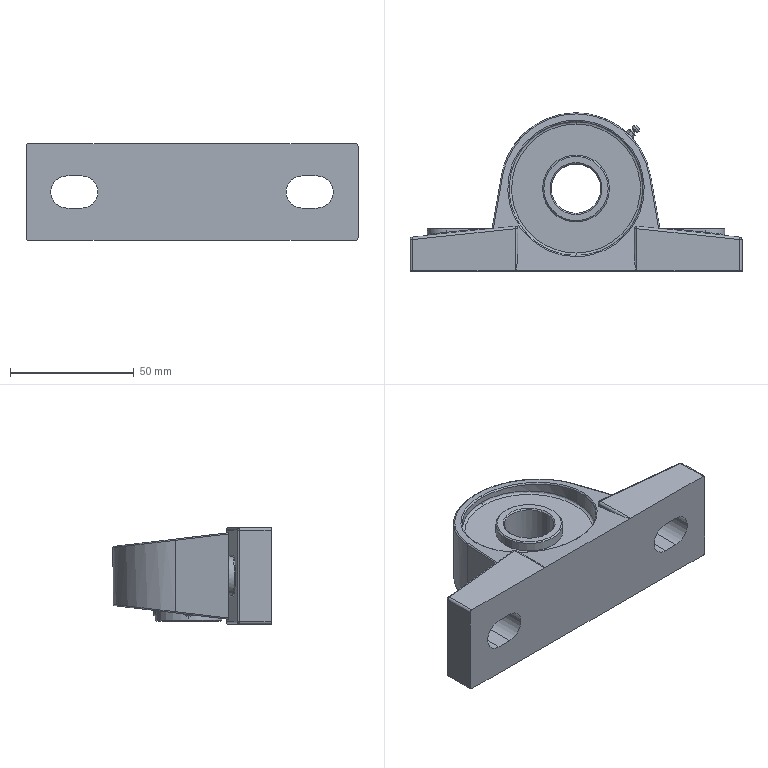Part | STEP file | 1 solid | 150 faces | box 134 x 63.85 x 39 mm | volume 118753 mm3 | cylinder 54 | plane 44 | cone 29 | spline 23 | commonest cylinder face diameters 2 x18 6 x9 1 x8 13 x4 27 x4 54.05 x4